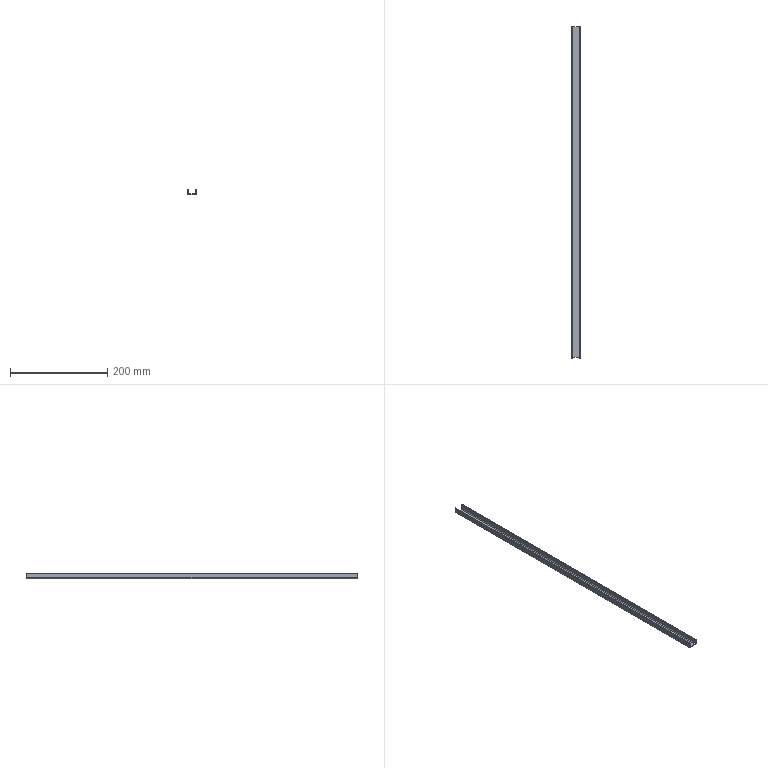Part | STEP file | Door reinforcing rib (flat door) modified U | 1 solid | 23 faces | box 20 x 684 x 12 mm | volume 51617 mm3 | plane 19 | cylinder 4 | commonest cylinder face diameters 3 x2 7 x2